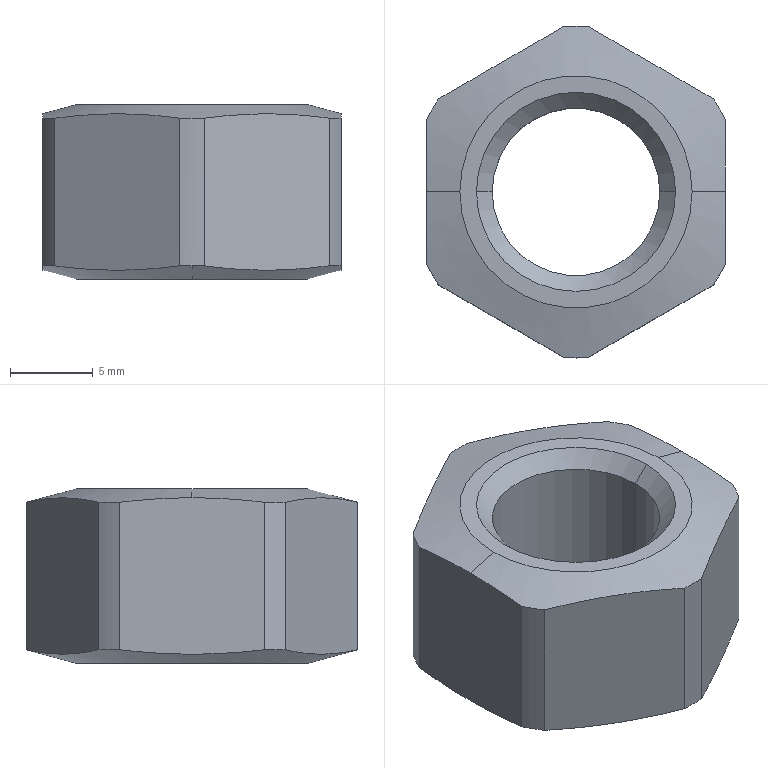Part | SolidWorks | features BaseBody 1 | 1 solid | 24 faces | box 18 x 20 x 10.5 mm | volume 1969 mm3 | cylinder 8 | cone 8 | plane 8 | commonest cylinder face diameters 20 x6 10.106 x2
STEP:
#1=CARTESIAN_POINT('',(-5.053,0.,-4.303));
#2=VERTEX_POINT('',#1);
#3=CARTESIAN_POINT('',(5.053,0.,-4.303));
#4=VERTEX_POINT('',#3);
#5=CARTESIAN_POINT('',(0.,0.,-4.303));
#6=DIRECTION('',(0.,0.,1.));
#7=DIRECTION('',(1.,0.,0.));
#8=AXIS2_PLACEMENT_3D('',#5,#6,#7);
#9=CIRCLE('',#8,5.053);
#10=EDGE_CURVE('',#2,#4,#9,.T.);
#11=ORIENTED_EDGE('',*,*,#10,.F.);
#12=CARTESIAN_POINT('',(-5.053,0.,4.303));
#13=VERTEX_POINT('',#12);
#14=CARTESIAN_POINT('',(-5.053,0.,-5.25));
#15=DIRECTION('',(0.,0.,1.));
#16=VECTOR('',#15,1000.);
#17=LINE('',#14,#16);
#18=EDGE_CURVE('',#2,#13,#17,.T.);
#19=ORIENTED_EDGE('',*,*,#18,.T.);
#20=CARTESIAN_POINT('',(5.053,0.,4.303));
#21=VERTEX_POINT('',#20);
#22=CARTESIAN_POINT('',(0.,0.,4.303));
#23=DIRECTION('',(0.,0.,-1.));
#24=DIRECTION('',(1.,0.,0.));
#25=AXIS2_PLACEMENT_3D('',#22,#23,#24);
#26=CIRCLE('',#25,5.053);
#27=EDGE_CURVE('',#21,#13,#26,.T.);
#28=ORIENTED_EDGE('',*,*,#27,.F.);
#29=CARTESIAN_POINT('',(5.053,0.,-5.25));
#30=DIRECTION('',(0.,0.,1.));
#31=VECTOR('',#30,1000.);
#32=LINE('',#29,#31);
#33=EDGE_CURVE('',#4,#21,#32,.T.);
#34=ORIENTED_EDGE('',*,*,#33,.F.);
#35=EDGE_LOOP('',(#11,#19,#28,#34));
#36=FACE_OUTER_BOUND('',#35,.T.);
#37=CARTESIAN_POINT('',(0.,0.,-5.25));
#38=DIRECTION('',(0.,0.,1.));
#39=DIRECTION('',(1.,0.,0.));
#40=AXIS2_PLACEMENT_3D('',#37,#38,#39);
#41=CYLINDRICAL_SURFACE('',#40,5.053);
#42=ADVANCED_FACE('',(#36),#41,.F.);
#43=ORIENTED_EDGE('',*,*,#27,.T.);
#44=CARTESIAN_POINT('',(-6.,0.,5.25));
#45=VERTEX_POINT('',#44);
#46=CARTESIAN_POINT('',(-6.,0.,5.25));
#47=DIRECTION('',(-0.7071,0.,0.7071));
#48=VECTOR('',#47,1000.);
#49=LINE('',#46,#48);
#50=EDGE_CURVE('',#13,#45,#49,.T.);
#51=ORIENTED_EDGE('',*,*,#50,.T.);
#52=CARTESIAN_POINT('',(6.,0.,5.25));
#53=VERTEX_POINT('',#52);
#54=CARTESIAN_POINT('',(0.,0.,5.25));
#55=DIRECTION('',(0.,0.,-1.));
#56=DIRECTION('',(1.,0.,0.));
#57=AXIS2_PLACEMENT_3D('',#54,#55,#56);
#58=CIRCLE('',#57,6.);
#59=EDGE_CURVE('',#53,#45,#58,.T.);
#60=ORIENTED_EDGE('',*,*,#59,.F.);
#61=CARTESIAN_POINT('',(6.,0.,5.25));
#62=DIRECTION('',(0.7071,0.,0.7071));
#63=VECTOR('',#62,1000.);
#64=LINE('',#61,#63);
#65=EDGE_CURVE('',#21,#53,#64,.T.);
#66=ORIENTED_EDGE('',*,*,#65,.F.);
#67=EDGE_LOOP('',(#43,#51,#60,#66));
#68=FACE_OUTER_BOUND('',#67,.T.);
#69=CARTESIAN_POINT('',(0.,0.,5.25));
#70=DIRECTION('',(0.,0.,1.));
#71=DIRECTION('',(1.,0.,0.));
#72=AXIS2_PLACEMENT_3D('',#69,#70,#71);
#73=CONICAL_SURFACE('',#72,6.,0.7854);
#74=ADVANCED_FACE('',(#68),#73,.F.);
#75=ORIENTED_EDGE('',*,*,#10,.T.);
#76=CARTESIAN_POINT('',(6.,0.,-5.25));
#77=VERTEX_POINT('',#76);
#78=CARTESIAN_POINT('',(6.,0.,-5.25));
#79=DIRECTION('',(0.7071,0.,-0.7071));
#80=VECTOR('',#79,1000.);
#81=LINE('',#78,#80);
#82=EDGE_CURVE('',#4,#77,#81,.T.);
#83=ORIENTED_EDGE('',*,*,#82,.T.);
#84=CARTESIAN_POINT('',(-6.,0.,-5.25));
#85=VERTEX_POINT('',#84);
#86=CARTESIAN_POINT('',(0.,0.,-5.25));
#87=DIRECTION('',(0.,0.,1.));
#88=DIRECTION('',(-1.,0.,0.));
#89=AXIS2_PLACEMENT_3D('',#86,#87,#88);
#90=CIRCLE('',#89,6.);
#91=EDGE_CURVE('',#85,#77,#90,.T.);
#92=ORIENTED_EDGE('',*,*,#91,.F.);
#93=CARTESIAN_POINT('',(-6.,0.,-5.25));
#94=DIRECTION('',(-0.7071,0.,-0.7071));
#95=VECTOR('',#94,1000.);
#96=LINE('',#93,#95);
#97=EDGE_CURVE('',#2,#85,#96,.T.);
#98=ORIENTED_EDGE('',*,*,#97,.F.);
#99=EDGE_LOOP('',(#75,#83,#92,#98));
#100=FACE_OUTER_BOUND('',#99,.T.);
#101=CARTESIAN_POINT('',(0.,0.,-5.25));
#102=DIRECTION('',(0.,0.,-1.));
#103=DIRECTION('',(-1.,0.,0.));
#104=AXIS2_PLACEMENT_3D('',#101,#102,#103);
#105=CONICAL_SURFACE('',#104,6.,0.7854);
#106=ADVANCED_FACE('',(#100),#105,.F.);
#107=CARTESIAN_POINT('',(-7.,0.,5.25));
#108=VERTEX_POINT('',#107);
#109=CARTESIAN_POINT('',(7.,0.,5.25));
#110=VERTEX_POINT('',#109);
#111=CARTESIAN_POINT('',(0.,0.,5.25));
#112=DIRECTION('',(0.,0.,-1.));
#113=DIRECTION('',(-1.,0.,0.));
#114=AXIS2_PLACEMENT_3D('',#111,#112,#113);
#115=CIRCLE('',#114,7.);
#116=EDGE_CURVE('',#108,#110,#115,.T.);
#117=ORIENTED_EDGE('',*,*,#116,.T.);
#118=CARTESIAN_POINT('',(9.,0.,4.714));
#119=VERTEX_POINT('',#118);
#120=CARTESIAN_POINT('',(10.,0.,4.446));
#121=DIRECTION('',(0.9659,0.,-0.2588));
#122=VECTOR('',#121,1000.);
#123=LINE('',#120,#122);
#124=EDGE_CURVE('',#110,#119,#123,.T.);
#125=ORIENTED_EDGE('',*,*,#124,.T.);
#126=CARTESIAN_POINT('',(9.,4.359,4.446));
#127=VERTEX_POINT('',#126);
#128=CARTESIAN_POINT('',(9.,0.,4.714));
#129=CARTESIAN_POINT('',(9.,1.453,4.714));
#130=CARTESIAN_POINT('',(9.,2.906,4.616));
#131=CARTESIAN_POINT('',(9.,4.359,4.446));
#132=B_SPLINE_CURVE_WITH_KNOTS('',3,(#128,#129,#130,#131),.UNSPECIFIED.,.F.,.F.,(4,4),(0.004359,0.008718),.UNSPECIFIED.);
#133=EDGE_CURVE('',#119,#127,#132,.T.);
#134=ORIENTED_EDGE('',*,*,#133,.T.);
#135=CARTESIAN_POINT('',(8.275,5.615,4.446));
#136=VERTEX_POINT('',#135);
#137=CARTESIAN_POINT('',(0.,0.,4.446));
#138=DIRECTION('',(0.,0.,-1.));
#139=DIRECTION('',(1.,0.,0.));
#140=AXIS2_PLACEMENT_3D('',#137,#138,#139);
#141=CIRCLE('',#140,10.);
#142=EDGE_CURVE('',#136,#127,#141,.T.);
#143=ORIENTED_EDGE('',*,*,#142,.F.);
#144=CARTESIAN_POINT('',(0.7251,9.974,4.446));
#145=VERTEX_POINT('',#144);
#146=CARTESIAN_POINT('',(8.275,5.615,4.446));
#147=CARTESIAN_POINT('',(7.017,6.341,4.616));
#148=CARTESIAN_POINT('',(4.5,7.794,4.812));
#149=CARTESIAN_POINT('',(1.983,9.247,4.616));
#150=CARTESIAN_POINT('',(0.7251,9.974,4.446));
#151=B_SPLINE_CURVE_WITH_KNOTS('',3,(#146,#147,#148,#149,#150),.UNSPECIFIED.,.F.,.F.,(4,1,4),(0.,0.004359,0.008718),.UNSPECIFIED.);
#152=EDGE_CURVE('',#136,#145,#151,.T.);
#153=ORIENTED_EDGE('',*,*,#152,.T.);
#154=CARTESIAN_POINT('',(-0.7251,9.974,4.446));
#155=VERTEX_POINT('',#154);
#156=CARTESIAN_POINT('',(0.,0.,4.446));
#157=DIRECTION('',(0.,0.,-1.));
#158=DIRECTION('',(1.,0.,0.));
#159=AXIS2_PLACEMENT_3D('',#156,#157,#158);
#160=CIRCLE('',#159,10.);
#161=EDGE_CURVE('',#155,#145,#160,.T.);
#162=ORIENTED_EDGE('',*,*,#161,.F.);
#163=CARTESIAN_POINT('',(-8.275,5.615,4.446));
#164=VERTEX_POINT('',#163);
#165=CARTESIAN_POINT('',(-0.7251,9.974,4.446));
#166=CARTESIAN_POINT('',(-1.983,9.247,4.616));
#167=CARTESIAN_POINT('',(-4.5,7.794,4.812));
#168=CARTESIAN_POINT('',(-7.017,6.341,4.616));
#169=CARTESIAN_POINT('',(-8.275,5.615,4.446));
#170=B_SPLINE_CURVE_WITH_KNOTS('',3,(#165,#166,#167,#168,#169),.UNSPECIFIED.,.F.,.F.,(4,1,4),(0.,0.004359,0.008718),.UNSPECIFIED.);
#171=EDGE_CURVE('',#155,#164,#170,.T.);
#172=ORIENTED_EDGE('',*,*,#171,.T.);
#173=CARTESIAN_POINT('',(-9.,4.359,4.446));
#174=VERTEX_POINT('',#173);
#175=CARTESIAN_POINT('',(0.,0.,4.446));
#176=DIRECTION('',(0.,0.,-1.));
#177=DIRECTION('',(1.,0.,0.));
#178=AXIS2_PLACEMENT_3D('',#175,#176,#177);
#179=CIRCLE('',#178,10.);
#180=EDGE_CURVE('',#174,#164,#179,.T.);
#181=ORIENTED_EDGE('',*,*,#180,.F.);
#182=CARTESIAN_POINT('',(-9.,0.,4.714));
#183=VERTEX_POINT('',#182);
#184=CARTESIAN_POINT('',(-9.,4.359,4.446));
#185=CARTESIAN_POINT('',(-9.,2.906,4.616));
#186=CARTESIAN_POINT('',(-9.,1.453,4.714));
#187=CARTESIAN_POINT('',(-9.,0.,4.714));
#188=B_SPLINE_CURVE_WITH_KNOTS('',3,(#184,#185,#186,#187),.UNSPECIFIED.,.F.,.F.,(4,4),(0.,0.004359),.UNSPECIFIED.);
#189=EDGE_CURVE('',#174,#183,#188,.T.);
#190=ORIENTED_EDGE('',*,*,#189,.T.);
#191=CARTESIAN_POINT('',(-10.,0.,4.446));
#192=DIRECTION('',(-0.9659,0.,-0.2588));
#193=VECTOR('',#192,1000.);
#194=LINE('',#191,#193);
#195=EDGE_CURVE('',#108,#183,#194,.T.);
#196=ORIENTED_EDGE('',*,*,#195,.F.);
#197=EDGE_LOOP('',(#117,#125,#134,#143,#153,#162,#172,#181,#190,#196));
#198=FACE_OUTER_BOUND('',#197,.T.);
#199=CARTESIAN_POINT('',(0.,0.,4.446));
#200=DIRECTION('',(0.,0.,-1.));
#201=DIRECTION('',(-1.,0.,0.));
#202=AXIS2_PLACEMENT_3D('',#199,#200,#201);
#203=CONICAL_SURFACE('',#202,10.,1.309);
#204=ADVANCED_FACE('',(#198),#203,.T.);
#205=CARTESIAN_POINT('',(0.,-7.,-5.25));
#206=VERTEX_POINT('',#205);
#207=CARTESIAN_POINT('',(0.,7.,-5.25));
#208=VERTEX_POINT('',#207);
#209=CARTESIAN_POINT('',(0.,0.,-5.25));
#210=DIRECTION('',(0.,0.,1.));
#211=DIRECTION('',(0.,-1.,0.));
#212=AXIS2_PLACEMENT_3D('',#209,#210,#211);
#213=CIRCLE('',#212,7.);
#214=EDGE_CURVE('',#206,#208,#213,.T.);
#215=ORIENTED_EDGE('',*,*,#214,.T.);
#216=CARTESIAN_POINT('',(0.,10.,-4.446));
#217=VERTEX_POINT('',#216);
#218=CARTESIAN_POINT('',(0.,10.,-4.446));
#219=DIRECTION('',(0.,0.9659,0.2588));
#220=VECTOR('',#219,1000.);
#221=LINE('',#218,#220);
#222=EDGE_CURVE('',#208,#217,#221,.T.);
#223=ORIENTED_EDGE('',*,*,#222,.T.);
#224=CARTESIAN_POINT('',(0.7251,9.974,-4.446));
#225=VERTEX_POINT('',#224);
#226=CARTESIAN_POINT('',(0.,0.,-4.446));
#227=DIRECTION('',(0.,0.,1.));
#228=DIRECTION('',(1.,0.,0.));
#229=AXIS2_PLACEMENT_3D('',#226,#227,#228);
#230=CIRCLE('',#229,10.);
#231=EDGE_CURVE('',#225,#217,#230,.T.);
#232=ORIENTED_EDGE('',*,*,#231,.F.);
#233=CARTESIAN_POINT('',(8.275,5.615,-4.446));
#234=VERTEX_POINT('',#233);
#235=CARTESIAN_POINT('',(0.7251,9.974,-4.446));
#236=CARTESIAN_POINT('',(1.983,9.247,-4.616));
#237=CARTESIAN_POINT('',(4.5,7.794,-4.812));
#238=CARTESIAN_POINT('',(7.017,6.341,-4.616));
#239=CARTESIAN_POINT('',(8.275,5.615,-4.446));
#240=B_SPLINE_CURVE_WITH_KNOTS('',3,(#235,#236,#237,#238,#239),.UNSPECIFIED.,.F.,.F.,(4,1,4),(0.,0.004359,0.008718),.UNSPECIFIED.);
#241=EDGE_CURVE('',#225,#234,#240,.T.);
#242=ORIENTED_EDGE('',*,*,#241,.T.);
#243=CARTESIAN_POINT('',(9.,4.359,-4.446));
#244=VERTEX_POINT('',#243);
#245=CARTESIAN_POINT('',(0.,0.,-4.446));
#246=DIRECTION('',(0.,0.,1.));
#247=DIRECTION('',(1.,0.,0.));
#248=AXIS2_PLACEMENT_3D('',#245,#246,#247);
#249=CIRCLE('',#248,10.);
#250=EDGE_CURVE('',#244,#234,#249,.T.);
#251=ORIENTED_EDGE('',*,*,#250,.F.);
#252=CARTESIAN_POINT('',(9.,-4.359,-4.446));
#253=VERTEX_POINT('',#252);
#254=CARTESIAN_POINT('',(9.,4.359,-4.446));
#255=CARTESIAN_POINT('',(9.,2.906,-4.616));
#256=CARTESIAN_POINT('',(9.,0.,-4.812));
#257=CARTESIAN_POINT('',(9.,-2.906,-4.616));
#258=CARTESIAN_POINT('',(9.,-4.359,-4.446));
#259=B_SPLINE_CURVE_WITH_KNOTS('',3,(#254,#255,#256,#257,#258),.UNSPECIFIED.,.F.,.F.,(4,1,4),(0.,0.004359,0.008718),.UNSPECIFIED.);
#260=EDGE_CURVE('',#244,#253,#259,.T.);
#261=ORIENTED_EDGE('',*,*,#260,.T.);
#262=CARTESIAN_POINT('',(8.275,-5.615,-4.446));
#263=VERTEX_POINT('',#262);
#264=CARTESIAN_POINT('',(0.,0.,-4.446));
#265=DIRECTION('',(0.,0.,1.));
#266=DIRECTION('',(1.,0.,0.));
#267=AXIS2_PLACEMENT_3D('',#264,#265,#266);
#268=CIRCLE('',#267,10.);
#269=EDGE_CURVE('',#263,#253,#268,.T.);
#270=ORIENTED_EDGE('',*,*,#269,.F.);
#271=CARTESIAN_POINT('',(0.7251,-9.974,-4.446));
#272=VERTEX_POINT('',#271);
#273=CARTESIAN_POINT('',(8.275,-5.615,-4.446));
#274=CARTESIAN_POINT('',(7.017,-6.341,-4.616));
#275=CARTESIAN_POINT('',(4.5,-7.794,-4.812));
#276=CARTESIAN_POINT('',(1.983,-9.247,-4.616));
#277=CARTESIAN_POINT('',(0.7251,-9.974,-4.446));
#278=B_SPLINE_CURVE_WITH_KNOTS('',3,(#273,#274,#275,#276,#277),.UNSPECIFIED.,.F.,.F.,(4,1,4),(0.,0.004359,0.008718),.UNSPECIFIED.);
#279=EDGE_CURVE('',#263,#272,#278,.T.);
#280=ORIENTED_EDGE('',*,*,#279,.T.);
#281=CARTESIAN_POINT('',(0.,-10.,-4.446));
#282=VERTEX_POINT('',#281);
#283=CARTESIAN_POINT('',(0.,0.,-4.446));
#284=DIRECTION('',(0.,0.,1.));
#285=DIRECTION('',(1.,0.,0.));
#286=AXIS2_PLACEMENT_3D('',#283,#284,#285);
#287=CIRCLE('',#286,10.);
#288=EDGE_CURVE('',#282,#272,#287,.T.);
#289=ORIENTED_EDGE('',*,*,#288,.F.);
#290=CARTESIAN_POINT('',(0.,-10.,-4.446));
#291=DIRECTION('',(0.,-0.9659,0.2588));
#292=VECTOR('',#291,1000.);
#293=LINE('',#290,#292);
#294=EDGE_CURVE('',#206,#282,#293,.T.);
#295=ORIENTED_EDGE('',*,*,#294,.F.);
#296=EDGE_LOOP('',(#215,#223,#232,#242,#251,#261,#270,#280,#289,#295));
#297=FACE_OUTER_BOUND('',#296,.T.);
#298=CARTESIAN_POINT('',(0.,0.,-4.446));
#299=DIRECTION('',(0.,0.,1.));
#300=DIRECTION('',(0.,-1.,0.));
#301=AXIS2_PLACEMENT_3D('',#298,#299,#300);
#302=CONICAL_SURFACE('',#301,10.,1.309);
#303=ADVANCED_FACE('',(#297),#302,.T.);
#304=ORIENTED_EDGE('',*,*,#18,.F.);
#305=CARTESIAN_POINT('',(0.,0.,-4.303));
#306=DIRECTION('',(0.,0.,1.));
#307=DIRECTION('',(1.,0.,0.));
#308=AXIS2_PLACEMENT_3D('',#305,#306,#307);
#309=CIRCLE('',#308,5.053);
#310=EDGE_CURVE('',#4,#2,#309,.T.);
#311=ORIENTED_EDGE('',*,*,#310,.F.);
#312=ORIENTED_EDGE('',*,*,#33,.T.);
#313=CARTESIAN_POINT('',(0.,0.,4.303));
#314=DIRECTION('',(0.,0.,-1.));
#315=DIRECTION('',(1.,0.,0.));
#316=AXIS2_PLACEMENT_3D('',#313,#314,#315);
#317=CIRCLE('',#316,5.053);
#318=EDGE_CURVE('',#13,#21,#317,.T.);
#319=ORIENTED_EDGE('',*,*,#318,.F.);
#320=EDGE_LOOP('',(#304,#311,#312,#319));
#321=FACE_OUTER_BOUND('',#320,.T.);
#322=CARTESIAN_POINT('',(0.,0.,-5.25));
#323=DIRECTION('',(0.,0.,1.));
#324=DIRECTION('',(1.,0.,0.));
#325=AXIS2_PLACEMENT_3D('',#322,#323,#324);
#326=CYLINDRICAL_SURFACE('',#325,5.053);
#327=ADVANCED_FACE('',(#321),#326,.F.);
#328=ORIENTED_EDGE('',*,*,#50,.F.);
#329=ORIENTED_EDGE('',*,*,#318,.T.);
#330=ORIENTED_EDGE('',*,*,#65,.T.);
#331=CARTESIAN_POINT('',(0.,0.,5.25));
#332=DIRECTION('',(0.,0.,-1.));
#333=DIRECTION('',(1.,0.,0.));
#334=AXIS2_PLACEMENT_3D('',#331,#332,#333);
#335=CIRCLE('',#334,6.);
#336=EDGE_CURVE('',#45,#53,#335,.T.);
#337=ORIENTED_EDGE('',*,*,#336,.F.);
#338=EDGE_LOOP('',(#328,#329,#330,#337));
#339=FACE_OUTER_BOUND('',#338,.T.);
#340=CARTESIAN_POINT('',(0.,0.,5.25));
#341=DIRECTION('',(0.,0.,1.));
#342=DIRECTION('',(1.,0.,0.));
#343=AXIS2_PLACEMENT_3D('',#340,#341,#342);
#344=CONICAL_SURFACE('',#343,6.,0.7854);
#345=ADVANCED_FACE('',(#339),#344,.F.);
#346=ORIENTED_EDGE('',*,*,#82,.F.);
#347=ORIENTED_EDGE('',*,*,#310,.T.);
#348=ORIENTED_EDGE('',*,*,#97,.T.);
#349=CARTESIAN_POINT('',(0.,0.,-5.25));
#350=DIRECTION('',(0.,0.,1.));
#351=DIRECTION('',(-1.,0.,0.));
#352=AXIS2_PLACEMENT_3D('',#349,#350,#351);
#353=CIRCLE('',#352,6.);
#354=EDGE_CURVE('',#77,#85,#353,.T.);
#355=ORIENTED_EDGE('',*,*,#354,.F.);
#356=EDGE_LOOP('',(#346,#347,#348,#355));
#357=FACE_OUTER_BOUND('',#356,.T.);
#358=CARTESIAN_POINT('',(0.,0.,-5.25));
#359=DIRECTION('',(0.,0.,-1.));
#360=DIRECTION('',(-1.,0.,0.));
#361=AXIS2_PLACEMENT_3D('',#358,#359,#360);
#362=CONICAL_SURFACE('',#361,6.,0.7854);
#363=ADVANCED_FACE('',(#357),#362,.F.);
#364=ORIENTED_EDGE('',*,*,#59,.T.);
#365=ORIENTED_EDGE('',*,*,#336,.T.);
#366=EDGE_LOOP('',(#364,#365));
#367=FACE_BOUND('',#366,.T.);
#368=ORIENTED_EDGE('',*,*,#116,.F.);
#369=CARTESIAN_POINT('',(0.,0.,5.25));
#370=DIRECTION('',(0.,0.,-1.));
#371=DIRECTION('',(-1.,0.,0.));
#372=AXIS2_PLACEMENT_3D('',#369,#370,#371);
#373=CIRCLE('',#372,7.);
#374=EDGE_CURVE('',#110,#108,#373,.T.);
#375=ORIENTED_EDGE('',*,*,#374,.F.);
#376=EDGE_LOOP('',(#368,#375));
#377=FACE_OUTER_BOUND('',#376,.T.);
#378=CARTESIAN_POINT('',(0.,0.,5.25));
#379=DIRECTION('',(0.,0.,-1.));
#380=DIRECTION('',(-1.,0.,0.));
#381=AXIS2_PLACEMENT_3D('',#378,#379,#380);
#382=PLANE('',#381);
#383=ADVANCED_FACE('',(#367,#377),#382,.F.);
#384=ORIENTED_EDGE('',*,*,#214,.F.);
#385=CARTESIAN_POINT('',(0.,0.,-5.25));
#386=DIRECTION('',(0.,0.,1.));
#387=DIRECTION('',(0.,-1.,0.));
#388=AXIS2_PLACEMENT_3D('',#385,#386,#387);
#389=CIRCLE('',#388,7.);
#390=EDGE_CURVE('',#208,#206,#389,.T.);
#391=ORIENTED_EDGE('',*,*,#390,.F.);
#392=EDGE_LOOP('',(#384,#391));
#393=FACE_OUTER_BOUND('',#392,.T.);
#394=ORIENTED_EDGE('',*,*,#91,.T.);
#395=ORIENTED_EDGE('',*,*,#354,.T.);
#396=EDGE_LOOP('',(#394,#395));
#397=FACE_BOUND('',#396,.T.);
#398=CARTESIAN_POINT('',(0.,7.,-5.25));
#399=DIRECTION('',(0.,0.,1.));
#400=DIRECTION('',(1.,0.,0.));
#401=AXIS2_PLACEMENT_3D('',#398,#399,#400);
#402=PLANE('',#401);
#403=ADVANCED_FACE('',(#393,#397),#402,.F.);
#404=ORIENTED_EDGE('',*,*,#124,.F.);
#405=ORIENTED_EDGE('',*,*,#374,.T.);
#406=ORIENTED_EDGE('',*,*,#195,.T.);
#407=CARTESIAN_POINT('',(-9.,-4.359,4.446));
#408=VERTEX_POINT('',#407);
#409=CARTESIAN_POINT('',(-9.,0.,4.714));
#410=CARTESIAN_POINT('',(-9.,-1.453,4.714));
#411=CARTESIAN_POINT('',(-9.,-2.906,4.616));
#412=CARTESIAN_POINT('',(-9.,-4.359,4.446));
#413=B_SPLINE_CURVE_WITH_KNOTS('',3,(#409,#410,#411,#412),.UNSPECIFIED.,.F.,.F.,(4,4),(0.004359,0.008718),.UNSPECIFIED.);
#414=EDGE_CURVE('',#183,#408,#413,.T.);
#415=ORIENTED_EDGE('',*,*,#414,.T.);
#416=CARTESIAN_POINT('',(-8.275,-5.615,4.446));
#417=VERTEX_POINT('',#416);
#418=CARTESIAN_POINT('',(0.,0.,4.446));
#419=DIRECTION('',(0.,0.,-1.));
#420=DIRECTION('',(1.,0.,0.));
#421=AXIS2_PLACEMENT_3D('',#418,#419,#420);
#422=CIRCLE('',#421,10.);
#423=EDGE_CURVE('',#417,#408,#422,.T.);
#424=ORIENTED_EDGE('',*,*,#423,.F.);
#425=CARTESIAN_POINT('',(-0.7251,-9.974,4.446));
#426=VERTEX_POINT('',#425);
#427=CARTESIAN_POINT('',(-8.275,-5.615,4.446));
#428=CARTESIAN_POINT('',(-7.017,-6.341,4.616));
#429=CARTESIAN_POINT('',(-4.5,-7.794,4.812));
#430=CARTESIAN_POINT('',(-1.983,-9.247,4.616));
#431=CARTESIAN_POINT('',(-0.7251,-9.974,4.446));
#432=B_SPLINE_CURVE_WITH_KNOTS('',3,(#427,#428,#429,#430,#431),.UNSPECIFIED.,.F.,.F.,(4,1,4),(0.,0.004359,0.008718),.UNSPECIFIED.);
#433=EDGE_CURVE('',#417,#426,#432,.T.);
#434=ORIENTED_EDGE('',*,*,#433,.T.);
#435=CARTESIAN_POINT('',(0.7251,-9.974,4.446));
#436=VERTEX_POINT('',#435);
#437=CARTESIAN_POINT('',(0.,0.,4.446));
#438=DIRECTION('',(0.,0.,-1.));
#439=DIRECTION('',(1.,0.,0.));
#440=AXIS2_PLACEMENT_3D('',#437,#438,#439);
#441=CIRCLE('',#440,10.);
#442=EDGE_CURVE('',#436,#426,#441,.T.);
#443=ORIENTED_EDGE('',*,*,#442,.F.);
#444=CARTESIAN_POINT('',(8.275,-5.615,4.446));
#445=VERTEX_POINT('',#444);
#446=CARTESIAN_POINT('',(0.7251,-9.974,4.446));
#447=CARTESIAN_POINT('',(1.983,-9.247,4.616));
#448=CARTESIAN_POINT('',(4.5,-7.794,4.812));
#449=CARTESIAN_POINT('',(7.017,-6.341,4.616));
#450=CARTESIAN_POINT('',(8.275,-5.615,4.446));
#451=B_SPLINE_CURVE_WITH_KNOTS('',3,(#446,#447,#448,#449,#450),.UNSPECIFIED.,.F.,.F.,(4,1,4),(0.,0.004359,0.008718),.UNSPECIFIED.);
#452=EDGE_CURVE('',#436,#445,#451,.T.);
#453=ORIENTED_EDGE('',*,*,#452,.T.);
#454=CARTESIAN_POINT('',(9.,-4.359,4.446));
#455=VERTEX_POINT('',#454);
#456=CARTESIAN_POINT('',(0.,0.,4.446));
#457=DIRECTION('',(0.,0.,-1.));
#458=DIRECTION('',(1.,0.,0.));
#459=AXIS2_PLACEMENT_3D('',#456,#457,#458);
#460=CIRCLE('',#459,10.);
#461=EDGE_CURVE('',#455,#445,#460,.T.);
#462=ORIENTED_EDGE('',*,*,#461,.F.);
#463=CARTESIAN_POINT('',(9.,-4.359,4.446));
#464=CARTESIAN_POINT('',(9.,-2.906,4.616));
#465=CARTESIAN_POINT('',(9.,-1.453,4.714));
#466=CARTESIAN_POINT('',(9.,0.,4.714));
#467=B_SPLINE_CURVE_WITH_KNOTS('',3,(#463,#464,#465,#466),.UNSPECIFIED.,.F.,.F.,(4,4),(0.,0.004359),.UNSPECIFIED.);
#468=EDGE_CURVE('',#455,#119,#467,.T.);
#469=ORIENTED_EDGE('',*,*,#468,.T.);
#470=EDGE_LOOP('',(#404,#405,#406,#415,#424,#434,#443,#453,#462,#469));
#471=FACE_OUTER_BOUND('',#470,.T.);
#472=CARTESIAN_POINT('',(0.,0.,4.446));
#473=DIRECTION('',(0.,0.,-1.));
#474=DIRECTION('',(-1.,0.,0.));
#475=AXIS2_PLACEMENT_3D('',#472,#473,#474);
#476=CONICAL_SURFACE('',#475,10.,1.309);
#477=ADVANCED_FACE('',(#471),#476,.T.);
#478=ORIENTED_EDGE('',*,*,#222,.F.);
#479=ORIENTED_EDGE('',*,*,#390,.T.);
#480=ORIENTED_EDGE('',*,*,#294,.T.);
#481=CARTESIAN_POINT('',(-0.7251,-9.974,-4.446));
#482=VERTEX_POINT('',#481);
#483=CARTESIAN_POINT('',(0.,0.,-4.446));
#484=DIRECTION('',(0.,0.,1.));
#485=DIRECTION('',(1.,0.,0.));
#486=AXIS2_PLACEMENT_3D('',#483,#484,#485);
#487=CIRCLE('',#486,10.);
#488=EDGE_CURVE('',#482,#282,#487,.T.);
#489=ORIENTED_EDGE('',*,*,#488,.F.);
#490=CARTESIAN_POINT('',(-8.275,-5.615,-4.446));
#491=VERTEX_POINT('',#490);
#492=CARTESIAN_POINT('',(-0.7251,-9.974,-4.446));
#493=CARTESIAN_POINT('',(-1.983,-9.247,-4.616));
#494=CARTESIAN_POINT('',(-4.5,-7.794,-4.812));
#495=CARTESIAN_POINT('',(-7.017,-6.341,-4.616));
#496=CARTESIAN_POINT('',(-8.275,-5.615,-4.446));
#497=B_SPLINE_CURVE_WITH_KNOTS('',3,(#492,#493,#494,#495,#496),.UNSPECIFIED.,.F.,.F.,(4,1,4),(0.,0.004359,0.008718),.UNSPECIFIED.);
#498=EDGE_CURVE('',#482,#491,#497,.T.);
#499=ORIENTED_EDGE('',*,*,#498,.T.);
#500=CARTESIAN_POINT('',(-9.,-4.359,-4.446));
#501=VERTEX_POINT('',#500);
#502=CARTESIAN_POINT('',(0.,0.,-4.446));
#503=DIRECTION('',(0.,0.,1.));
#504=DIRECTION('',(1.,0.,0.));
#505=AXIS2_PLACEMENT_3D('',#502,#503,#504);
#506=CIRCLE('',#505,10.);
#507=EDGE_CURVE('',#501,#491,#506,.T.);
#508=ORIENTED_EDGE('',*,*,#507,.F.);
#509=CARTESIAN_POINT('',(-9.,4.359,-4.446));
#510=VERTEX_POINT('',#509);
#511=CARTESIAN_POINT('',(-9.,-4.359,-4.446));
#512=CARTESIAN_POINT('',(-9.,-2.906,-4.616));
#513=CARTESIAN_POINT('',(-9.,0.,-4.812));
#514=CARTESIAN_POINT('',(-9.,2.906,-4.616));
#515=CARTESIAN_POINT('',(-9.,4.359,-4.446));
#516=B_SPLINE_CURVE_WITH_KNOTS('',3,(#511,#512,#513,#514,#515),.UNSPECIFIED.,.F.,.F.,(4,1,4),(0.,0.004359,0.008718),.UNSPECIFIED.);
#517=EDGE_CURVE('',#501,#510,#516,.T.);
#518=ORIENTED_EDGE('',*,*,#517,.T.);
#519=CARTESIAN_POINT('',(-8.275,5.615,-4.446));
#520=VERTEX_POINT('',#519);
#521=CARTESIAN_POINT('',(0.,0.,-4.446));
#522=DIRECTION('',(0.,0.,1.));
#523=DIRECTION('',(1.,0.,0.));
#524=AXIS2_PLACEMENT_3D('',#521,#522,#523);
#525=CIRCLE('',#524,10.);
#526=EDGE_CURVE('',#520,#510,#525,.T.);
#527=ORIENTED_EDGE('',*,*,#526,.F.);
#528=CARTESIAN_POINT('',(-0.7251,9.974,-4.446));
#529=VERTEX_POINT('',#528);
#530=CARTESIAN_POINT('',(-8.275,5.615,-4.446));
#531=CARTESIAN_POINT('',(-7.017,6.341,-4.616));
#532=CARTESIAN_POINT('',(-4.5,7.794,-4.812));
#533=CARTESIAN_POINT('',(-1.983,9.247,-4.616));
#534=CARTESIAN_POINT('',(-0.7251,9.974,-4.446));
#535=B_SPLINE_CURVE_WITH_KNOTS('',3,(#530,#531,#532,#533,#534),.UNSPECIFIED.,.F.,.F.,(4,1,4),(0.,0.004359,0.008718),.UNSPECIFIED.);
#536=EDGE_CURVE('',#520,#529,#535,.T.);
#537=ORIENTED_EDGE('',*,*,#536,.T.);
#538=CARTESIAN_POINT('',(0.,0.,-4.446));
#539=DIRECTION('',(0.,0.,1.));
#540=DIRECTION('',(1.,0.,0.));
#541=AXIS2_PLACEMENT_3D('',#538,#539,#540);
#542=CIRCLE('',#541,10.);
#543=EDGE_CURVE('',#217,#529,#542,.T.);
#544=ORIENTED_EDGE('',*,*,#543,.F.);
#545=EDGE_LOOP('',(#478,#479,#480,#489,#499,#508,#518,#527,#537,#544));
#546=FACE_OUTER_BOUND('',#545,.T.);
#547=CARTESIAN_POINT('',(0.,0.,-4.446));
#548=DIRECTION('',(0.,0.,1.));
#549=DIRECTION('',(0.,-1.,0.));
#550=AXIS2_PLACEMENT_3D('',#547,#548,#549);
#551=CONICAL_SURFACE('',#550,10.,1.309);
#552=ADVANCED_FACE('',(#546),#551,.T.);
#553=CARTESIAN_POINT('',(0.7251,9.974,5.25));
#554=DIRECTION('',(0.,0.,-1.));
#555=VECTOR('',#554,1000.);
#556=LINE('',#553,#555);
#557=EDGE_CURVE('',#145,#225,#556,.T.);
#558=ORIENTED_EDGE('',*,*,#557,.F.);
#559=ORIENTED_EDGE('',*,*,#152,.F.);
#560=CARTESIAN_POINT('',(8.275,5.615,5.25));
#561=DIRECTION('',(0.,0.,1.));
#562=VECTOR('',#561,1000.);
#563=LINE('',#560,#562);
#564=EDGE_CURVE('',#234,#136,#563,.T.);
#565=ORIENTED_EDGE('',*,*,#564,.F.);
#566=ORIENTED_EDGE('',*,*,#241,.F.);
#567=EDGE_LOOP('',(#558,#559,#565,#566));
#568=FACE_OUTER_BOUND('',#567,.T.);
#569=CARTESIAN_POINT('',(9.,5.196,5.25));
#570=DIRECTION('',(-0.5,-0.866,0.));
#571=DIRECTION('',(0.866,-0.5,0.));
#572=AXIS2_PLACEMENT_3D('',#569,#570,#571);
#573=PLANE('',#572);
#574=ADVANCED_FACE('',(#568),#573,.F.);
#575=CARTESIAN_POINT('',(9.,4.359,5.25));
#576=DIRECTION('',(0.,0.,-1.));
#577=VECTOR('',#576,1000.);
#578=LINE('',#575,#577);
#579=EDGE_CURVE('',#127,#244,#578,.T.);
#580=ORIENTED_EDGE('',*,*,#579,.F.);
#581=ORIENTED_EDGE('',*,*,#133,.F.);
#582=ORIENTED_EDGE('',*,*,#468,.F.);
#583=CARTESIAN_POINT('',(9.,-4.359,5.25));
#584=DIRECTION('',(0.,0.,1.));
#585=VECTOR('',#584,1000.);
#586=LINE('',#583,#585);
#587=EDGE_CURVE('',#253,#455,#586,.T.);
#588=ORIENTED_EDGE('',*,*,#587,.F.);
#589=ORIENTED_EDGE('',*,*,#260,.F.);
#590=EDGE_LOOP('',(#580,#581,#582,#588,#589));
#591=FACE_OUTER_BOUND('',#590,.T.);
#592=CARTESIAN_POINT('',(9.,-5.196,5.25));
#593=DIRECTION('',(-1.,0.,0.));
#594=DIRECTION('',(0.,0.,1.));
#595=AXIS2_PLACEMENT_3D('',#592,#593,#594);
#596=PLANE('',#595);
#597=ADVANCED_FACE('',(#591),#596,.F.);
#598=CARTESIAN_POINT('',(8.275,-5.615,5.25));
#599=DIRECTION('',(0.,0.,-1.));
#600=VECTOR('',#599,1000.);
#601=LINE('',#598,#600);
#602=EDGE_CURVE('',#445,#263,#601,.T.);
#603=ORIENTED_EDGE('',*,*,#602,.F.);
#604=ORIENTED_EDGE('',*,*,#452,.F.);
#605=CARTESIAN_POINT('',(0.7251,-9.974,5.25));
#606=DIRECTION('',(0.,0.,1.));
#607=VECTOR('',#606,1000.);
#608=LINE('',#605,#607);
#609=EDGE_CURVE('',#272,#436,#608,.T.);
#610=ORIENTED_EDGE('',*,*,#609,.F.);
#611=ORIENTED_EDGE('',*,*,#279,.F.);
#612=EDGE_LOOP('',(#603,#604,#610,#611));
#613=FACE_OUTER_BOUND('',#612,.T.);
#614=CARTESIAN_POINT('',(0.,-10.392,5.25));
#615=DIRECTION('',(-0.5,0.866,0.));
#616=DIRECTION('',(-0.866,-0.5,0.));
#617=AXIS2_PLACEMENT_3D('',#614,#615,#616);
#618=PLANE('',#617);
#619=ADVANCED_FACE('',(#613),#618,.F.);
#620=CARTESIAN_POINT('',(-0.7251,-9.974,5.25));
#621=DIRECTION('',(0.,0.,-1.));
#622=VECTOR('',#621,1000.);
#623=LINE('',#620,#622);
#624=EDGE_CURVE('',#426,#482,#623,.T.);
#625=ORIENTED_EDGE('',*,*,#624,.F.);
#626=ORIENTED_EDGE('',*,*,#433,.F.);
#627=CARTESIAN_POINT('',(-8.275,-5.615,5.25));
#628=DIRECTION('',(0.,0.,1.));
#629=VECTOR('',#628,1000.);
#630=LINE('',#627,#629);
#631=EDGE_CURVE('',#491,#417,#630,.T.);
#632=ORIENTED_EDGE('',*,*,#631,.F.);
#633=ORIENTED_EDGE('',*,*,#498,.F.);
#634=EDGE_LOOP('',(#625,#626,#632,#633));
#635=FACE_OUTER_BOUND('',#634,.T.);
#636=CARTESIAN_POINT('',(-9.,-5.196,5.25));
#637=DIRECTION('',(0.5,0.866,0.));
#638=DIRECTION('',(-0.866,0.5,0.));
#639=AXIS2_PLACEMENT_3D('',#636,#637,#638);
#640=PLANE('',#639);
#641=ADVANCED_FACE('',(#635),#640,.F.);
#642=CARTESIAN_POINT('',(-9.,-4.359,5.25));
#643=DIRECTION('',(0.,0.,-1.));
#644=VECTOR('',#643,1000.);
#645=LINE('',#642,#644);
#646=EDGE_CURVE('',#408,#501,#645,.T.);
#647=ORIENTED_EDGE('',*,*,#646,.F.);
#648=ORIENTED_EDGE('',*,*,#414,.F.);
#649=ORIENTED_EDGE('',*,*,#189,.F.);
#650=CARTESIAN_POINT('',(-9.,4.359,5.25));
#651=DIRECTION('',(0.,0.,1.));
#652=VECTOR('',#651,1000.);
#653=LINE('',#650,#652);
#654=EDGE_CURVE('',#510,#174,#653,.T.);
#655=ORIENTED_EDGE('',*,*,#654,.F.);
#656=ORIENTED_EDGE('',*,*,#517,.F.);
#657=EDGE_LOOP('',(#647,#648,#649,#655,#656));
#658=FACE_OUTER_BOUND('',#657,.T.);
#659=CARTESIAN_POINT('',(-9.,5.196,5.25));
#660=DIRECTION('',(1.,0.,0.));
#661=DIRECTION('',(0.,0.,-1.));
#662=AXIS2_PLACEMENT_3D('',#659,#660,#661);
#663=PLANE('',#662);
#664=ADVANCED_FACE('',(#658),#663,.F.);
#665=CARTESIAN_POINT('',(-8.275,5.615,5.25));
#666=DIRECTION('',(0.,0.,-1.));
#667=VECTOR('',#666,1000.);
#668=LINE('',#665,#667);
#669=EDGE_CURVE('',#164,#520,#668,.T.);
#670=ORIENTED_EDGE('',*,*,#669,.F.);
#671=ORIENTED_EDGE('',*,*,#171,.F.);
#672=CARTESIAN_POINT('',(-0.7251,9.974,5.25));
#673=DIRECTION('',(0.,0.,1.));
#674=VECTOR('',#673,1000.);
#675=LINE('',#672,#674);
#676=EDGE_CURVE('',#529,#155,#675,.T.);
#677=ORIENTED_EDGE('',*,*,#676,.F.);
#678=ORIENTED_EDGE('',*,*,#536,.F.);
#679=EDGE_LOOP('',(#670,#671,#677,#678));
#680=FACE_OUTER_BOUND('',#679,.T.);
#681=CARTESIAN_POINT('',(0.,10.392,5.25));
#682=DIRECTION('',(0.5,-0.866,0.));
#683=DIRECTION('',(0.866,0.5,0.));
#684=AXIS2_PLACEMENT_3D('',#681,#682,#683);
#685=PLANE('',#684);
#686=ADVANCED_FACE('',(#680),#685,.F.);
#687=ORIENTED_EDGE('',*,*,#676,.T.);
#688=ORIENTED_EDGE('',*,*,#161,.T.);
#689=ORIENTED_EDGE('',*,*,#557,.T.);
#690=ORIENTED_EDGE('',*,*,#231,.T.);
#691=ORIENTED_EDGE('',*,*,#543,.T.);
#692=EDGE_LOOP('',(#687,#688,#689,#690,#691));
#693=FACE_OUTER_BOUND('',#692,.T.);
#694=CARTESIAN_POINT('',(0.,0.,5.25));
#695=DIRECTION('',(0.,0.,1.));
#696=DIRECTION('',(1.,0.,0.));
#697=AXIS2_PLACEMENT_3D('',#694,#695,#696);
#698=CYLINDRICAL_SURFACE('',#697,10.);
#699=ADVANCED_FACE('',(#693),#698,.T.);
#700=ORIENTED_EDGE('',*,*,#564,.T.);
#701=ORIENTED_EDGE('',*,*,#142,.T.);
#702=ORIENTED_EDGE('',*,*,#579,.T.);
#703=ORIENTED_EDGE('',*,*,#250,.T.);
#704=EDGE_LOOP('',(#700,#701,#702,#703));
#705=FACE_OUTER_BOUND('',#704,.T.);
#706=CARTESIAN_POINT('',(0.,0.,5.25));
#707=DIRECTION('',(0.,0.,1.));
#708=DIRECTION('',(1.,0.,0.));
#709=AXIS2_PLACEMENT_3D('',#706,#707,#708);
#710=CYLINDRICAL_SURFACE('',#709,10.);
#711=ADVANCED_FACE('',(#705),#710,.T.);
#712=ORIENTED_EDGE('',*,*,#587,.T.);
#713=ORIENTED_EDGE('',*,*,#461,.T.);
#714=ORIENTED_EDGE('',*,*,#602,.T.);
#715=ORIENTED_EDGE('',*,*,#269,.T.);
#716=EDGE_LOOP('',(#712,#713,#714,#715));
#717=FACE_OUTER_BOUND('',#716,.T.);
#718=CARTESIAN_POINT('',(0.,0.,5.25));
#719=DIRECTION('',(0.,0.,1.));
#720=DIRECTION('',(1.,0.,0.));
#721=AXIS2_PLACEMENT_3D('',#718,#719,#720);
#722=CYLINDRICAL_SURFACE('',#721,10.);
#723=ADVANCED_FACE('',(#717),#722,.T.);
#724=ORIENTED_EDGE('',*,*,#609,.T.);
#725=ORIENTED_EDGE('',*,*,#442,.T.);
#726=ORIENTED_EDGE('',*,*,#624,.T.);
#727=ORIENTED_EDGE('',*,*,#488,.T.);
#728=ORIENTED_EDGE('',*,*,#288,.T.);
#729=EDGE_LOOP('',(#724,#725,#726,#727,#728));
#730=FACE_OUTER_BOUND('',#729,.T.);
#731=CARTESIAN_POINT('',(0.,0.,5.25));
#732=DIRECTION('',(0.,0.,1.));
#733=DIRECTION('',(1.,0.,0.));
#734=AXIS2_PLACEMENT_3D('',#731,#732,#733);
#735=CYLINDRICAL_SURFACE('',#734,10.);
#736=ADVANCED_FACE('',(#730),#735,.T.);
#737=ORIENTED_EDGE('',*,*,#631,.T.);
#738=ORIENTED_EDGE('',*,*,#423,.T.);
#739=ORIENTED_EDGE('',*,*,#646,.T.);
#740=ORIENTED_EDGE('',*,*,#507,.T.);
#741=EDGE_LOOP('',(#737,#738,#739,#740));
#742=FACE_OUTER_BOUND('',#741,.T.);
#743=CARTESIAN_POINT('',(0.,0.,5.25));
#744=DIRECTION('',(0.,0.,1.));
#745=DIRECTION('',(1.,0.,0.));
#746=AXIS2_PLACEMENT_3D('',#743,#744,#745);
#747=CYLINDRICAL_SURFACE('',#746,10.);
#748=ADVANCED_FACE('',(#742),#747,.T.);
#749=ORIENTED_EDGE('',*,*,#654,.T.);
#750=ORIENTED_EDGE('',*,*,#180,.T.);
#751=ORIENTED_EDGE('',*,*,#669,.T.);
#752=ORIENTED_EDGE('',*,*,#526,.T.);
#753=EDGE_LOOP('',(#749,#750,#751,#752));
#754=FACE_OUTER_BOUND('',#753,.T.);
#755=CARTESIAN_POINT('',(0.,0.,5.25));
#756=DIRECTION('',(0.,0.,1.));
#757=DIRECTION('',(1.,0.,0.));
#758=AXIS2_PLACEMENT_3D('',#755,#756,#757);
#759=CYLINDRICAL_SURFACE('',#758,10.);
#760=ADVANCED_FACE('',(#754),#759,.T.);
#761=CLOSED_SHELL('',(#42,#74,#106,#204,#303,#327,#345,#363,#383,#403,#477,#552,#574,#597,#619,#641,#664,#686,#699,#711,#723,#736,#748,#760));
#762=MANIFOLD_SOLID_BREP('',#761);
#763=CARTESIAN_POINT('',(0.,0.,0.));
#764=DIRECTION('',(0.,0.,1.));
#765=DIRECTION('',(1.,0.,0.));
#766=AXIS2_PLACEMENT_3D('',#763,#764,#765);
#767=(LENGTH_UNIT()NAMED_UNIT(*)SI_UNIT(.MILLI.,.METRE.));
#768=UNCERTAINTY_MEASURE_WITH_UNIT(LENGTH_MEASURE(0.00001),#767,'','');
#769=(NAMED_UNIT(*)PLANE_ANGLE_UNIT()SI_UNIT($,.RADIAN.));
#770=(NAMED_UNIT(*)SI_UNIT($,.STERADIAN.)SOLID_ANGLE_UNIT());
#771=(GEOMETRIC_REPRESENTATION_CONTEXT(3)GLOBAL_UNCERTAINTY_ASSIGNED_CONTEXT((#768))GLOBAL_UNIT_ASSIGNED_CONTEXT((#767,#769,#770))REPRESENTATION_CONTEXT('',''));
#772=ADVANCED_BREP_SHAPE_REPRESENTATION('',(#762,#766),#771);